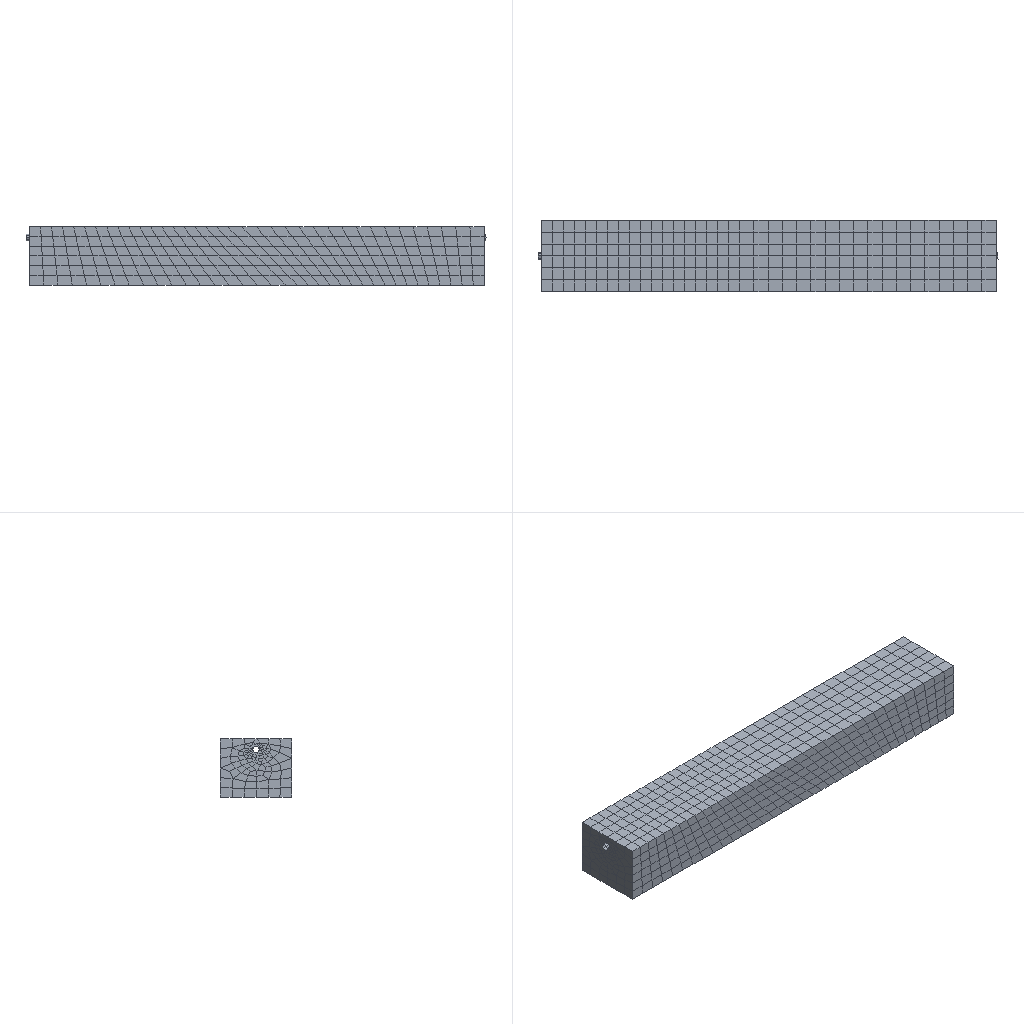Simulation study | abaqus
Set-up summary:
category,name,step,type,value,unit,region
solver,abaqus
solver,version,,,Abaqus/Standard 2020
units,not stated in the deck,,not stated
analysis,deck,,transient,transient
load_step,Step-1,Step-1,transient,nlgeom=True
load_step,Step-p,Step-p,transient,nlgeom=True
load_step,Step-u,Step-u,transient,nlgeom=True
contact,interactions,,,general=1 pairs=0 ties=0
load_step,requested,,,3
mesh,nodes,,,5780
mesh,elements,,,4784
element_type,S4R,,shell,680
element_type,C3D8R,,solid,4104
load,load commands in deck,,count,3
bc,support commands in deck,,count,9
material,SOIL,,in results
material,TUBE,,in results
check,setup vs results,,match,"per instance, exact: element labels, types and connectivity; labels of the nodes the elements use; coordinates not compared"
Abaqus input file, long lists of numbers shortened:
*Heading
** Job name: Job-1 Model name: Model-1
** Generated by: Abaqus/CAE 2020
*Preprint, echo=NO, model=NO, history=NO, contact=NO
**
** PARTS
**
*Part, name=Part-1
*Node
      1,  0.431,         84.5, -0.431
      2,           0.,         84.5, -0.6095
** (686 more lines like these left out)
*Element, type=S4R
  1,   8,   1,   9,  16
  2,   1,   2,  10,   9
** (678 more lines like these left out)
*Nset, nset=Set-2, generate
   1,  688,    1
*Elset, elset=Set-2, generate
   1,  680,    1
** Section: Section-1
*Shell Section, elset=Set-2, material=tube
0.0264, 5
*End Part
**
*Part, name=soil-m2
*Node
      1,   38.055,  -6.873,   9.345
      2,   38.209,  -7.067,    9.191
** (2563 more lines like these left out)
*Element, type=C3D8R
   1,  121,   45,    1,   43,  256,  180,  136,  178
   2,   48,  117,    4,    3,  183,  252,  139,  138
** (2068 more lines like these left out)
*Nset, nset=Set-1, generate
    1,  2565,     1
*Elset, elset=Set-1, generate
    1,  2070,     1
** Section: soil
*Solid Section, elset=Set-1, material=soil
,
*End Part
**
*Part, name=soil-m11
*Node
      1,   38.055,  -6.327,   9.345
      2,   38.209,  -6.133,    9.191
** (2525 more lines like these left out)
*Element, type=C3D8R
   1,   16,  119,   45,    1,  149,  252,  178,  134
   2,   48,  117,    4,    3,  181,  250,  137,  136
** (2032 more lines like these left out)
*Nset, nset=Set-1, generate
    1,  2527,     1
*Elset, elset=Set-1, generate
    1,  2034,     1
** Section: soil
*Solid Section, elset=Set-1, material=soil
,
*End Part
**
**
** ASSEMBLY
**
*Assembly, name=Assembly
**
*Instance, name=Part-1-1, part=Part-1
      83.835,         -6.6,          8.8
      83.835,         -6.6,          8.8,       83.835,         -6.6, 9.8, 90.
*End Instance
**
*Instance, name=soil-m11-1, part=soil-m11
*End Instance
**
*Instance, name=soil-m2-1, part=soil-m2
*End Instance
**
*Nset, nset=Set-1, instance=soil-m11-1
   21,   22,   34,   35,   36,   37,   38,  154,  155,  167,  168,  169,  170,  171,  287,  288
  300,  301,  302,  303,  304,  420,  421,  433,  434,  435,  436,  437,  553,  554,  566,  567
** (7 more lines like these left out)
*Nset, nset=Set-1, instance=soil-m2-1
   17,   19,   25,   26,   27,   28,   29,  152,  154,  160,  161,  162,  163,  164,  287,  289
  295,  296,  297,  298,  299,  422,  424,  430,  431,  432,  433,  434,  557,  559,  565,  566
** (7 more lines like these left out)
*Elset, elset=Set-1, instance=soil-m11-1
   25,   26,   31,  101,  102,  103,  138,  139,  144,  214,  215,  216,  251,  252,  257,  327
  328,  329,  364,  365,  370,  440,  441,  442,  477,  478,  483,  553,  554,  555,  590,  591
** (5 more lines like these left out)
*Elset, elset=Set-1, instance=soil-m2-1
   17,   18,   19,   22,   93,  104,  132,  133,  134,  137,  208,  219,  247,  248,  249,  252
  323,  334,  362,  363,  364,  367,  438,  449,  477,  478,  479,  482,  553,  564,  592,  593
** (5 more lines like these left out)
*Nset, nset=Set-2, instance=soil-m11-1
   17,   18,   19,   20,   21,   22,   23,   24,   30,   31,   32,   33,   39,   40,  150,  151
  152,  153,  154,  155,  156,  157,  163,  164,  165,  166,  172,  173,  283,  284,  285,  286
** (15 more lines like these left out)
*Nset, nset=Set-2, instance=soil-m2-1
   17,   18,   19,   20,   21,   22,   23,   24,   30,   31,   32,   33,   39,   40,  152,  153
  154,  155,  156,  157,  158,  159,  165,  166,  167,  168,  174,  175,  287,  288,  289,  290
** (15 more lines like these left out)
*Elset, elset=Set-2, instance=soil-m11-1
   16,   19,   22,   26,   30,   31,   77,   85,   88,   93,   98,  104,  129,  132,  135,  139
  143,  144,  190,  198,  201,  206,  211,  217,  242,  245,  248,  252,  256,  257,  303,  311
** (12 more lines like these left out)
*Elset, elset=Set-2, instance=soil-m2-1
   17,   18,   24,   25,   27,   88,   89,   91,   94,   96,   98,  103,  132,  133,  139,  140
  142,  203,  204,  206,  209,  211,  213,  218,  247,  248,  254,  255,  257,  318,  319,  321
** (12 more lines like these left out)
*Nset, nset=Set-3, instance=soil-m11-1, generate
 2395,  2527,     1
*Nset, nset=Set-3, instance=soil-m2-1, generate
 2431,  2565,     1
*Elset, elset=Set-3, instance=soil-m11-1, generate
 1922,  2034,     1
*Elset, elset=Set-3, instance=soil-m2-1, generate
 1956,  2070,     1
*Nset, nset=Set-4, instance=soil-m2-1
   21,   22,   34,   35,   36,   37,   38,  156,  157,  169,  170,  171,  172,  173,  291,  292
  304,  305,  306,  307,  308,  426,  427,  439,  440,  441,  442,  443,  561,  562,  574,  575
** (7 more lines like these left out)
*Elset, elset=Set-4, instance=soil-m2-1
   25,   27,   53,   75,   76,   77,  140,  142,  168,  190,  191,  192,  255,  257,  283,  305
  306,  307,  370,  372,  398,  420,  421,  422,  485,  487,  513,  535,  536,  537,  600,  602
** (5 more lines like these left out)
*Nset, nset=Set-5, instance=soil-m11-1
   21,   22,   34,   35,   36,   37,   38,  154,  155,  167,  168,  169,  170,  171,  287,  288
  300,  301,  302,  303,  304,  420,  421,  433,  434,  435,  436,  437,  553,  554,  566,  567
** (7 more lines like these left out)
*Elset, elset=Set-5, instance=soil-m11-1
   25,   26,   31,  101,  102,  103,  138,  139,  144,  214,  215,  216,  251,  252,  257,  327
  328,  329,  364,  365,  370,  440,  441,  442,  477,  478,  483,  553,  554,  555,  590,  591
** (5 more lines like these left out)
*Nset, nset=Set-6, instance=soil-m11-1
   17,   18,   19,   20,   21,   22,   23,   24,   30,   31,   32,   33,   39,   40,  150,  151
  152,  153,  154,  155,  156,  157,  163,  164,  165,  166,  172,  173,  283,  284,  285,  286
** (15 more lines like these left out)
*Elset, elset=Set-6, instance=soil-m11-1
   16,   19,   22,   26,   30,   31,   77,   85,   88,   93,   98,  104,  129,  132,  135,  139
  143,  144,  190,  198,  201,  206,  211,  217,  242,  245,  248,  252,  256,  257,  303,  311
** (12 more lines like these left out)
*Nset, nset=Set-7, instance=soil-m11-1, generate
 2395,  2527,     1
*Elset, elset=Set-7, instance=soil-m11-1, generate
 1922,  2034,     1
*Elset, elset=_Surf-3_SPOS, internal, instance=Part-1-1, generate
   1,  680,    1
*Surface, type=ELEMENT, name=Surf-3
_Surf-3_SPOS, SPOS
*Elset, elset=_m_Surf-1_SNEG, internal, instance=Part-1-1, generate
   1,  680,    1
*Surface, type=ELEMENT, name=m_Surf-1
_m_Surf-1_SNEG, SNEG
*Elset, elset=_m_Surf-4_E4, internal, instance=Part-1-1, generate
   1,  673,    8
*Surface, type=ELEMENT, name=m_Surf-4
_m_Surf-4_E4, E4
*Elset, elset=_m_Surf-6_SNEG, internal, instance=Part-1-1, generate
   1,  680,    1
*Surface, type=ELEMENT, name=m_Surf-6
_m_Surf-6_SNEG, SNEG
*Elset, elset=_m_Surf-8_S1, internal, instance=soil-m11-1, generate
   1,  113,    1
*Surface, type=ELEMENT, name=m_Surf-8
_m_Surf-8_S1, S1
*Elset, elset=_m_Surf-10_SNEG, internal, instance=Part-1-1, generate
   1,  680,    1
*Surface, type=ELEMENT, name=m_Surf-10
_m_Surf-10_SNEG, SNEG
*Elset, elset=_s_Surf-1_S6, internal, instance=soil-m11-1
    1,   13,   18,   20,  114,  126,  131,  133,  227,  239,  244,  246,  340,  352,  357,  359
  453,  465,  470,  472,  566,  578,  583,  585,  679,  691,  696,  698,  792,  804,  809,  811
** (3 more lines like these left out)
*Elset, elset=_s_Surf-1_S5, internal, instance=soil-m11-1, generate
    2,  1923,   113
*Elset, elset=_s_Surf-1_S5, internal, instance=soil-m2-1
    2,    8,   23,  117,  123,  138,  232,  238,  253,  347,  353,  368,  462,  468,  483,  577
  583,  598,  692,  698,  713,  807,  813,  828,  922,  928,  943, 1037, 1043, 1058, 1152, 1158
** (2 more lines like these left out)
*Elset, elset=_s_Surf-1_S4, internal, instance=soil-m11-1
   11,   32,   34,   36,   37,   39,  124,  145,  147,  149,  150,  152,  237,  258,  260,  262
  263,  265,  350,  371,  373,  375,  376,  378,  463,  484,  486,  488,  489,  491,  576,  597
** (5 more lines like these left out)
*Elset, elset=_s_Surf-1_S4, internal, instance=soil-m2-1
    3,   10,   34,   36,   37,   39,   42,  118,  125,  149,  151,  152,  154,  157,  233,  240
  264,  266,  267,  269,  272,  348,  355,  379,  381,  382,  384,  387,  463,  470,  494,  496
** (6 more lines like these left out)
*Elset, elset=_s_Surf-1_S3, internal, instance=soil-m11-1
   14,   15,   23,   35,   43,  127,  128,  136,  148,  156,  240,  241,  249,  261,  269,  353
  354,  362,  374,  382,  466,  467,  475,  487,  495,  579,  580,  588,  600,  608,  692,  693
** (4 more lines like these left out)
*Elset, elset=_s_Surf-1_S3, internal, instance=soil-m2-1
    7,   12,   13,   16,   35,   43,  122,  127,  128,  131,  150,  158,  237,  242,  243,  246
  265,  273,  352,  357,  358,  361,  380,  388,  467,  472,  473,  476,  495,  503,  582,  587
** (5 more lines like these left out)
*Surface, type=ELEMENT, name=s_Surf-1
_s_Surf-1_S6, S6
_s_Surf-1_S5, S5
_s_Surf-1_S4, S4
_s_Surf-1_S3, S3
*Elset, elset=_s_Surf-4_S6, internal, instance=soil-m11-1
    1,   13,   18,   20,  114,  126,  131,  133,  227,  239,  244,  246,  340,  352,  357,  359
  453,  465,  470,  472,  566,  578,  583,  585,  679,  691,  696,  698,  792,  804,  809,  811
** (3 more lines like these left out)
*Elset, elset=_s_Surf-4_S5, internal, instance=soil-m11-1, generate
    2,  1923,   113
*Elset, elset=_s_Surf-4_S5, internal, instance=soil-m2-1
    2,    8,   23,  117,  123,  138,  232,  238,  253,  347,  353,  368,  462,  468,  483,  577
  583,  598,  692,  698,  713,  807,  813,  828,  922,  928,  943, 1037, 1043, 1058, 1152, 1158
** (2 more lines like these left out)
*Elset, elset=_s_Surf-4_S4, internal, instance=soil-m11-1
   11,   32,   34,   36,   37,   39,  124,  145,  147,  149,  150,  152,  237,  258,  260,  262
  263,  265,  350,  371,  373,  375,  376,  378,  463,  484,  486,  488,  489,  491,  576,  597
** (5 more lines like these left out)
*Elset, elset=_s_Surf-4_S4, internal, instance=soil-m2-1
    3,   10,   34,   36,   37,   39,   42,  118,  125,  149,  151,  152,  154,  157,  233,  240
  264,  266,  267,  269,  272,  348,  355,  379,  381,  382,  384,  387,  463,  470,  494,  496
** (6 more lines like these left out)
*Elset, elset=_s_Surf-4_S3, internal, instance=soil-m11-1
   14,   15,   23,   35,   43,  127,  128,  136,  148,  156,  240,  241,  249,  261,  269,  353
  354,  362,  374,  382,  466,  467,  475,  487,  495,  579,  580,  588,  600,  608,  692,  693
** (4 more lines like these left out)
*Elset, elset=_s_Surf-4_S3, internal, instance=soil-m2-1
    7,   12,   13,   16,   35,   43,  122,  127,  128,  131,  150,  158,  237,  242,  243,  246
  265,  273,  352,  357,  358,  361,  380,  388,  467,  472,  473,  476,  495,  503,  582,  587
** (5 more lines like these left out)
*Surface, type=ELEMENT, name=s_Surf-4
_s_Surf-4_S6, S6
_s_Surf-4_S5, S5
_s_Surf-4_S4, S4
_s_Surf-4_S3, S3
*Elset, elset=_s_Surf-6_S6, internal, instance=soil-m11-1
    1,   13,   18,   20,  114,  126,  131,  133,  227,  239,  244,  246,  340,  352,  357,  359
  453,  465,  470,  472,  566,  578,  583,  585,  679,  691,  696,  698,  792,  804,  809,  811
** (3 more lines like these left out)
*Elset, elset=_s_Surf-6_S5, internal, instance=soil-m11-1, generate
    2,  1923,   113
*Elset, elset=_s_Surf-6_S5, internal, instance=soil-m2-1
    2,    8,   23,  117,  123,  138,  232,  238,  253,  347,  353,  368,  462,  468,  483,  577
  583,  598,  692,  698,  713,  807,  813,  828,  922,  928,  943, 1037, 1043, 1058, 1152, 1158
** (2 more lines like these left out)
*Elset, elset=_s_Surf-6_S4, internal, instance=soil-m11-1
   11,   32,   34,   36,   37,   39,  124,  145,  147,  149,  150,  152,  237,  258,  260,  262
  263,  265,  350,  371,  373,  375,  376,  378,  463,  484,  486,  488,  489,  491,  576,  597
** (5 more lines like these left out)
*Elset, elset=_s_Surf-6_S4, internal, instance=soil-m2-1
    3,   10,   34,   36,   37,   39,   42,  118,  125,  149,  151,  152,  154,  157,  233,  240
  264,  266,  267,  269,  272,  348,  355,  379,  381,  382,  384,  387,  463,  470,  494,  496
** (6 more lines like these left out)
*Elset, elset=_s_Surf-6_S3, internal, instance=soil-m11-1
   14,   15,   23,   35,   43,  127,  128,  136,  148,  156,  240,  241,  249,  261,  269,  353
  354,  362,  374,  382,  466,  467,  475,  487,  495,  579,  580,  588,  600,  608,  692,  693
** (4 more lines like these left out)
*Elset, elset=_s_Surf-6_S3, internal, instance=soil-m2-1
    7,   12,   13,   16,   35,   43,  122,  127,  128,  131,  150,  158,  237,  242,  243,  246
  265,  273,  352,  357,  358,  361,  380,  388,  467,  472,  473,  476,  495,  503,  582,  587
** (5 more lines like these left out)
*Surface, type=ELEMENT, name=s_Surf-6
_s_Surf-6_S6, S6
_s_Surf-6_S5, S5
_s_Surf-6_S4, S4
_s_Surf-6_S3, S3
*Elset, elset=_s_Surf-8_S1, internal, instance=soil-m2-1, generate
   1,  115,    1
*Surface, type=ELEMENT, name=s_Surf-8
_s_Surf-8_S1, S1
*Elset, elset=_s_Surf-10_S6, internal, instance=soil-m11-1
    1,   13,   18,   20,  114,  126,  131,  133,  227,  239,  244,  246,  340,  352,  357,  359
  453,  465,  470,  472,  566,  578,  583,  585,  679,  691,  696,  698,  792,  804,  809,  811
** (3 more lines like these left out)
*Elset, elset=_s_Surf-10_S5, internal, instance=soil-m11-1, generate
    2,  1923,   113
*Elset, elset=_s_Surf-10_S5, internal, instance=soil-m2-1
    2,    8,   23,  117,  123,  138,  232,  238,  253,  347,  353,  368,  462,  468,  483,  577
  583,  598,  692,  698,  713,  807,  813,  828,  922,  928,  943, 1037, 1043, 1058, 1152, 1158
** (2 more lines like these left out)
*Elset, elset=_s_Surf-10_S4, internal, instance=soil-m11-1
   11,   32,   34,   36,   37,   39,  124,  145,  147,  149,  150,  152,  237,  258,  260,  262
  263,  265,  350,  371,  373,  375,  376,  378,  463,  484,  486,  488,  489,  491,  576,  597
** (5 more lines like these left out)
*Elset, elset=_s_Surf-10_S4, internal, instance=soil-m2-1
    3,   10,   34,   36,   37,   39,   42,  118,  125,  149,  151,  152,  154,  157,  233,  240
  264,  266,  267,  269,  272,  348,  355,  379,  381,  382,  384,  387,  463,  470,  494,  496
** (6 more lines like these left out)
*Elset, elset=_s_Surf-10_S3, internal, instance=soil-m11-1
   14,   15,   23,   35,   43,  127,  128,  136,  148,  156,  240,  241,  249,  261,  269,  353
  354,  362,  374,  382,  466,  467,  475,  487,  495,  579,  580,  588,  600,  608,  692,  693
** (4 more lines like these left out)
*Elset, elset=_s_Surf-10_S3, internal, instance=soil-m2-1
    7,   12,   13,   16,   35,   43,  122,  127,  128,  131,  150,  158,  237,  242,  243,  246
  265,  273,  352,  357,  358,  361,  380,  388,  467,  472,  473,  476,  495,  503,  582,  587
** (5 more lines like these left out)
*Surface, type=ELEMENT, name=s_Surf-10
_s_Surf-10_S6, S6
_s_Surf-10_S5, S5
_s_Surf-10_S4, S4
_s_Surf-10_S3, S3
*Elset, elset=__Int-3_gcs0_1_SPOS, internal, instance=Part-1-1, generate
   1,  680,    1
*Surface, type=ELEMENT, name=_Int-3_gcs0_1, internal
__Int-3_gcs0_1_SPOS, SPOS
*Elset, elset=__Int-3_gcs0_2_SNEG, internal, instance=Part-1-1, generate
   1,  680,    1
*Surface, type=ELEMENT, name=_Int-3_gcs0_2, internal
__Int-3_gcs0_2_SNEG, SNEG
*Elset, elset=__Int-3_gcs0_3_S6, internal, instance=soil-m11-1
    1,   13,   18,   20,  114,  126,  131,  133,  227,  239,  244,  246,  340,  352,  357,  359
  453,  465,  470,  472,  566,  578,  583,  585,  679,  691,  696,  698,  792,  804,  809,  811
** (3 more lines like these left out)
*Elset, elset=__Int-3_gcs0_3_S5, internal, instance=soil-m11-1, generate
    2,  1923,   113
*Elset, elset=__Int-3_gcs0_3_S4, internal, instance=soil-m11-1
   11,   32,   34,   36,   37,   39,  124,  145,  147,  149,  150,  152,  237,  258,  260,  262
  263,  265,  350,  371,  373,  375,  376,  378,  463,  484,  486,  488,  489,  491,  576,  597
** (5 more lines like these left out)
*Elset, elset=__Int-3_gcs0_3_S3, internal, instance=soil-m11-1
   14,   15,   23,   35,   43,  127,  128,  136,  148,  156,  240,  241,  249,  261,  269,  353
  354,  362,  374,  382,  466,  467,  475,  487,  495,  579,  580,  588,  600,  608,  692,  693
** (4 more lines like these left out)
*Surface, type=ELEMENT, name=_Int-3_gcs0_3, internal
__Int-3_gcs0_3_S6, S6
__Int-3_gcs0_3_S5, S5
__Int-3_gcs0_3_S4, S4
__Int-3_gcs0_3_S3, S3
*Elset, elset=__Int-3_gcs0_10_S5, internal, instance=soil-m2-1
    2,    8,   23,  117,  123,  138,  232,  238,  253,  347,  353,  368,  462,  468,  483,  577
  583,  598,  692,  698,  713,  807,  813,  828,  922,  928,  943, 1037, 1043, 1058, 1152, 1158
** (2 more lines like these left out)
*Elset, elset=__Int-3_gcs0_10_S4, internal, instance=soil-m2-1
    3,   10,   34,   36,   37,   39,   42,  118,  125,  149,  151,  152,  154,  157,  233,  240
  264,  266,  267,  269,  272,  348,  355,  379,  381,  382,  384,  387,  463,  470,  494,  496
** (6 more lines like these left out)
*Elset, elset=__Int-3_gcs0_10_S3, internal, instance=soil-m2-1
    7,   12,   13,   16,   35,   43,  122,  127,  128,  131,  150,  158,  237,  242,  243,  246
  265,  273,  352,  357,  358,  361,  380,  388,  467,  472,  473,  476,  495,  503,  582,  587
** (5 more lines like these left out)
*Surface, type=ELEMENT, name=_Int-3_gcs0_10, internal
__Int-3_gcs0_10_S5, S5
__Int-3_gcs0_10_S4, S4
__Int-3_gcs0_10_S3, S3
*End Assembly
*Amplitude, name=Amp-1
             0.,              0.,              1.,              1.
**
** MATERIALS
**
*Material, name=soil
*Density
1900.,
*Elastic
 4e+07, 0.35
*Mohr Coulomb
22., 0.1
*Mohr Coulomb Hardening
40000.,0.
*Material, name=tube
*Density
7800.,
*Elastic
 2.1e+11, 0.3
*Plastic
 5.2e+08,0.
**
** INTERACTION PROPERTIES
**
*Surface Interaction, name=IntProp-1
1.,
*Friction, slip tolerance=0.005
 0.2,
*Surface Behavior, pressure-overclosure=HARD
**
** INTERACTIONS
**
** Interaction: Int-3
*Contact
*Contact Inclusions, ALL EXTERIOR
*Contact Property Assignment
 ,  , IntProp-1
*Surface Property Assignment, property=GEOMETRIC CORRECTION
_Int-3_gcs0_1, Circumferential, 41.835, -6.6, 8.8,  42.835, -6.6, 8.8
_Int-3_gcs0_2, Circumferential, 41.835, -6.6, 8.8,  42.835, -6.6, 8.8
_Int-3_gcs0_3, Circumferential, -0.665, -6.6, 8.8,  0.335, -6.6, 8.8
_Int-3_gcs0_10, Circumferential, -0.665, -6.6, 8.8,  0.335, -6.6, 8.8
** ----------------------------------------------------------------
**
** STEP: Step-1
**
*Step, name=Step-1, nlgeom=YES, inc=1000
*Dynamic
0.01,1.,1e-05
**
** BOUNDARY CONDITIONS
**
** Name: BC-1 Type: 位移/转角
*Boundary
Set-1, 3, 3
** Name: BC-2 Type: 位移/转角
*Boundary
Set-2, 2, 2
** Name: BC-3 Type: 位移/转角
*Boundary
Set-3, 1, 1
**
** LOADS
**
** Name: Load-1   Type: Gravity
*Dload
, GRAV, 9.8, 0., 0., -1.
**
** OUTPUT REQUESTS
**
*Restart, write, frequency=0
**
** FIELD OUTPUT: F-Output-1
**
*Output, field, frequency=1
*Node Output
A, CF, RF, U, V
*Element Output, directions=YES
E, LE, MISES, MISESMAX, PE, PEEQ, PEMAG, S, SSAVG
*Contact Output
CDISP, CSTRESS
**
** HISTORY OUTPUT: H-Output-1
**
*Output, history, variable=PRESELECT, frequency=1
*End Step
** ----------------------------------------------------------------
**
** STEP: Step-p
**
*Step, name=Step-p, nlgeom=YES, inc=1000
*Dynamic
0.01,1.,1e-05
**
** LOADS
**
** Name: Load-2   Type: Pressure
*Dsload, amplitude=Amp-1
Surf-3, P, 1.2e+07
**
** OUTPUT REQUESTS
**
*Restart, write, frequency=0
**
** FIELD OUTPUT: F-Output-1
**
*Output, field, frequency=1
*Node Output
A, CF, RF, U, V
*Element Output, directions=YES
E, LE, MISES, MISESMAX, PE, PEEQ, PEMAG, S, SSAVG
*Contact Output
CDISP, CSTRESS
**
** HISTORY OUTPUT: H-Output-1
**
*Output, history, variable=PRESELECT, frequency=1
*End Step
** ----------------------------------------------------------------
**
** STEP: Step-u
**
*Step, name=Step-u, nlgeom=YES, inc=1000
*Dynamic
0.01,1.,1e-05
**
** BOUNDARY CONDITIONS
**
** Name: BC-1 Type: 位移/转角
*Boundary, op=NEW
Set-1, 3, 3
** Name: BC-2 Type: 位移/转角
*Boundary, op=NEW
Set-2, 2, 2
** Name: BC-3 Type: 位移/转角
*Boundary, op=NEW
** Name: BC-5 Type: 位移/转角
*Boundary, op=NEW
Set-5, 3, 3
** Name: BC-6 Type: 位移/转角
*Boundary, op=NEW
Set-6, 2, 2
** Name: BC-7 Type: 位移/转角
*Boundary, op=NEW
Set-7, 1, 1
** Name: [REDACTED] : Displacement/rotation angle
*Boundary, op=NEW, amplitude=Amp-1
Set-4, 3, 3, -1.
**
** OUTPUT REQUESTS
**
*Restart, write, frequency=0
**
** FIELD OUTPUT: F-Output-1
**
*Output, field, frequency=1
*Node Output
CF, RF, RT, U, V
*Element Output, directions=YES
E, LE, MISES, MISESMAX, PE, PEEQ, PEMAG, S, SSAVG, TSHR
*Contact Output
CDISP, CSTRESS
**
** HISTORY OUTPUT: H-Output-1
**
*Output, history, variable=PRESELECT, frequency=1
*End Step
Results summary:
result,step,,completed,increments=61 time=1.0/1.0
result,step,,completed,increments=73 time=1.0/1.0
result,step,,completed,increments=171 time=1.0/1.0
result,analysis,,,transient
result,last_loadstep,,,3
result,analysis steps,,count,3
result,primary field,,,"U, UR"
result,reaction total,,FX,34645595.297,model units
result,reaction total,,FY,-614880.601,model units
result,reaction total,,FZ,233476899.844,model units